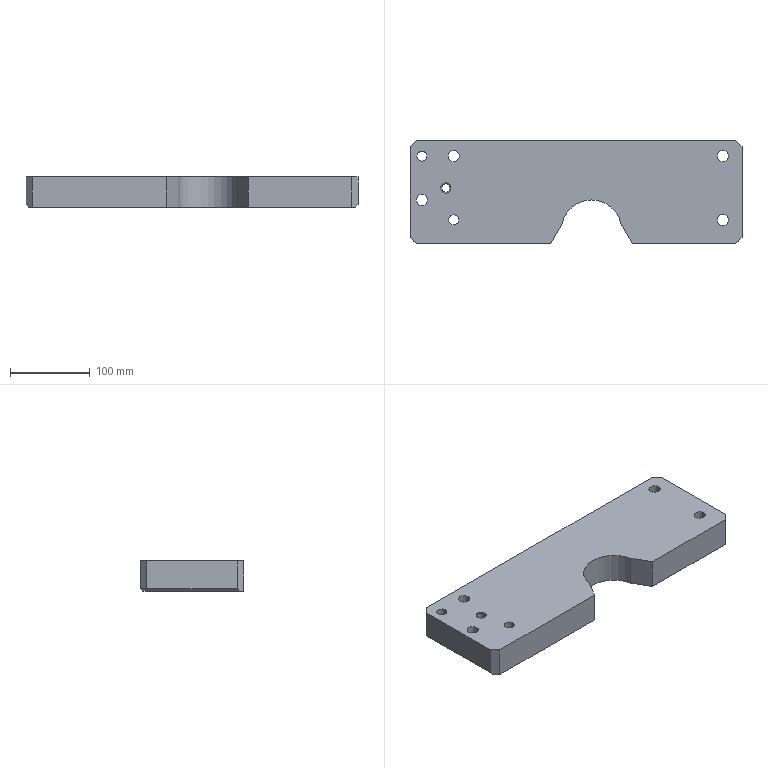Part | STEP file | 1_id950_x_t | 1 solid | 56 faces | box 417 x 130 x 38.1 mm | volume 1861233 mm3 | cylinder 29 | plane 25 | cone 2 | commonest cylinder face diameters 14 x14 20 x8 12.7 x4 10.716 x2 76.2 x1